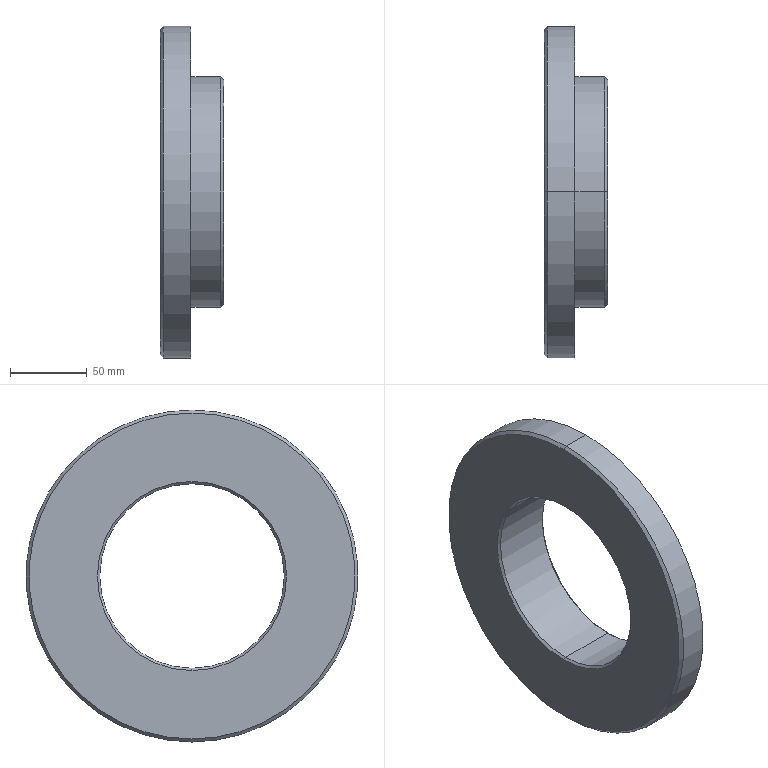Part | STEP file | Oil retaining ring | 1 solid | 17 faces | box 41.5 x 216 x 216 mm | volume 640315 mm3 | cone 8 | cylinder 6 | plane 3 | commonest cylinder face diameters 120 x2 150 x2 216 x2
STEP:
#1=CARTESIAN_POINT('',(0.,0.,0.));
#2=DIRECTION('',(0.,0.,1.));
#3=DIRECTION('',(1.,0.,0.));
#4=AXIS2_PLACEMENT_3D('',#1,#2,#3);
#5=CARTESIAN_POINT('',(39.5,0.,75.));
#6=VERTEX_POINT('',#5);
#7=CARTESIAN_POINT('',(39.5,0.,-75.));
#8=VERTEX_POINT('',#7);
#9=CARTESIAN_POINT('',(39.5,0.,0.));
#10=DIRECTION('',(-1.,0.,0.));
#11=DIRECTION('',(0.,0.,1.));
#12=AXIS2_PLACEMENT_3D('',#9,#10,#11);
#13=CIRCLE('',#12,75.);
#14=CARTESIAN_POINT('',(0.,0.,0.));
#15=DIRECTION('',(-1.,0.,0.));
#16=DIRECTION('',(0.,0.,1.));
#17=AXIS2_PLACEMENT_3D('',#14,#15,#16);
#18=CYLINDRICAL_SURFACE('',#17,75.);
#19=CARTESIAN_POINT('',(0.,-39.5));
#20=DIRECTION('',(1.,0.));
#21=VECTOR('',#20,1.);
#22=LINE('',#19,#21);
#23=(GEOMETRIC_REPRESENTATION_CONTEXT(2)PARAMETRIC_REPRESENTATION_CONTEXT()REPRESENTATION_CONTEXT('',''));
#24=DEFINITIONAL_REPRESENTATION('',(#22),#23);
#25=PCURVE('',#18,#24);
#26=CARTESIAN_POINT('',(41.5,0.,0.));
#27=DIRECTION('',(-1.,0.,0.));
#28=DIRECTION('',(0.,0.,1.));
#29=AXIS2_PLACEMENT_3D('',#26,#27,#28);
#30=CONICAL_SURFACE('',#29,73.,0.7854);
#31=CARTESIAN_POINT('',(0.,2.));
#32=DIRECTION('',(1.,0.));
#33=VECTOR('',#32,1.);
#34=LINE('',#31,#33);
#35=(GEOMETRIC_REPRESENTATION_CONTEXT(2)PARAMETRIC_REPRESENTATION_CONTEXT()REPRESENTATION_CONTEXT('',''));
#36=DEFINITIONAL_REPRESENTATION('',(#34),#35);
#37=PCURVE('',#30,#36);
#38=SURFACE_CURVE('',#13,(#25,#37),.PCURVE_S1.);
#39=EDGE_CURVE('',#6,#8,#38,.T.);
#40=ORIENTED_EDGE('',*,*,#39,.T.);
#41=CARTESIAN_POINT('',(20.,0.,-75.));
#42=VERTEX_POINT('',#41);
#43=CARTESIAN_POINT('',(0.,0.,-75.));
#44=DIRECTION('',(-1.,0.,0.));
#45=VECTOR('',#44,1.);
#46=LINE('',#43,#45);
#47=CARTESIAN_POINT('',(3.142,0.));
#48=DIRECTION('',(0.,1.));
#49=VECTOR('',#48,1.);
#50=LINE('',#47,#49);
#51=(GEOMETRIC_REPRESENTATION_CONTEXT(2)PARAMETRIC_REPRESENTATION_CONTEXT()REPRESENTATION_CONTEXT('',''));
#52=DEFINITIONAL_REPRESENTATION('',(#50),#51);
#53=PCURVE('',#18,#52);
#54=CARTESIAN_POINT('',(0.,0.,0.));
#55=DIRECTION('',(-1.,0.,0.));
#56=DIRECTION('',(0.,0.,1.));
#57=AXIS2_PLACEMENT_3D('',#54,#55,#56);
#58=CYLINDRICAL_SURFACE('',#57,75.);
#59=CARTESIAN_POINT('',(3.142,0.));
#60=DIRECTION('',(0.,1.));
#61=VECTOR('',#60,1.);
#62=LINE('',#59,#61);
#63=(GEOMETRIC_REPRESENTATION_CONTEXT(2)PARAMETRIC_REPRESENTATION_CONTEXT()REPRESENTATION_CONTEXT('',''));
#64=DEFINITIONAL_REPRESENTATION('',(#62),#63);
#65=PCURVE('',#58,#64);
#66=SURFACE_CURVE('',#46,(#53,#65),.PCURVE_S1.);
#67=EDGE_CURVE('',#8,#42,#66,.T.);
#68=ORIENTED_EDGE('',*,*,#67,.T.);
#69=CARTESIAN_POINT('',(20.,0.,75.));
#70=VERTEX_POINT('',#69);
#71=CARTESIAN_POINT('',(20.,0.,0.));
#72=DIRECTION('',(-1.,0.,0.));
#73=DIRECTION('',(0.,0.,1.));
#74=AXIS2_PLACEMENT_3D('',#71,#72,#73);
#75=CIRCLE('',#74,75.);
#76=CARTESIAN_POINT('',(0.,-20.));
#77=DIRECTION('',(1.,0.));
#78=VECTOR('',#77,1.);
#79=LINE('',#76,#78);
#80=(GEOMETRIC_REPRESENTATION_CONTEXT(2)PARAMETRIC_REPRESENTATION_CONTEXT()REPRESENTATION_CONTEXT('',''));
#81=DEFINITIONAL_REPRESENTATION('',(#79),#80);
#82=PCURVE('',#18,#81);
#83=CARTESIAN_POINT('',(20.,108.,0.));
#84=DIRECTION('',(-1.,0.,0.));
#85=DIRECTION('',(0.,0.,1.));
#86=AXIS2_PLACEMENT_3D('',#83,#84,#85);
#87=PLANE('',#86);
#88=CARTESIAN_POINT('',(0.,-108.));
#89=DIRECTION('',(1.,0.));
#90=AXIS2_PLACEMENT_2D('',#88,#89);
#91=CIRCLE('',#90,75.);
#92=(GEOMETRIC_REPRESENTATION_CONTEXT(2)PARAMETRIC_REPRESENTATION_CONTEXT()REPRESENTATION_CONTEXT('',''));
#93=DEFINITIONAL_REPRESENTATION('',(#91),#92);
#94=PCURVE('',#87,#93);
#95=SURFACE_CURVE('',#75,(#82,#94),.PCURVE_S1.);
#96=EDGE_CURVE('',#70,#42,#95,.T.);
#97=ORIENTED_EDGE('',*,*,#96,.F.);
#98=CARTESIAN_POINT('',(0.,0.,75.));
#99=DIRECTION('',(-1.,0.,0.));
#100=VECTOR('',#99,1.);
#101=LINE('',#98,#100);
#102=CARTESIAN_POINT('',(0.,0.));
#103=DIRECTION('',(0.,1.));
#104=VECTOR('',#103,1.);
#105=LINE('',#102,#104);
#106=(GEOMETRIC_REPRESENTATION_CONTEXT(2)PARAMETRIC_REPRESENTATION_CONTEXT()REPRESENTATION_CONTEXT('',''));
#107=DEFINITIONAL_REPRESENTATION('',(#105),#106);
#108=PCURVE('',#18,#107);
#109=CARTESIAN_POINT('',(6.283,0.));
#110=DIRECTION('',(0.,1.));
#111=VECTOR('',#110,1.);
#112=LINE('',#109,#111);
#113=(GEOMETRIC_REPRESENTATION_CONTEXT(2)PARAMETRIC_REPRESENTATION_CONTEXT()REPRESENTATION_CONTEXT('',''));
#114=DEFINITIONAL_REPRESENTATION('',(#112),#113);
#115=PCURVE('',#58,#114);
#116=SURFACE_CURVE('',#101,(#108,#115),.PCURVE_S1.);
#117=EDGE_CURVE('',#6,#70,#116,.T.);
#118=ORIENTED_EDGE('',*,*,#117,.F.);
#119=EDGE_LOOP('',(#40,#68,#97,#118));
#120=FACE_BOUND('',#119,.T.);
#121=ADVANCED_FACE('',(#120),#18,.T.);
#122=CARTESIAN_POINT('',(20.,0.,108.));
#123=VERTEX_POINT('',#122);
#124=CARTESIAN_POINT('',(20.,0.,-108.));
#125=VERTEX_POINT('',#124);
#126=CARTESIAN_POINT('',(20.,0.,0.));
#127=DIRECTION('',(-1.,0.,0.));
#128=DIRECTION('',(0.,0.,1.));
#129=AXIS2_PLACEMENT_3D('',#126,#127,#128);
#130=CIRCLE('',#129,108.);
#131=CARTESIAN_POINT('',(0.,0.,0.));
#132=DIRECTION('',(-1.,0.,0.));
#133=DIRECTION('',(0.,0.,1.));
#134=AXIS2_PLACEMENT_3D('',#131,#132,#133);
#135=CYLINDRICAL_SURFACE('',#134,108.);
#136=CARTESIAN_POINT('',(0.,-20.));
#137=DIRECTION('',(1.,0.));
#138=VECTOR('',#137,1.);
#139=LINE('',#136,#138);
#140=(GEOMETRIC_REPRESENTATION_CONTEXT(2)PARAMETRIC_REPRESENTATION_CONTEXT()REPRESENTATION_CONTEXT('',''));
#141=DEFINITIONAL_REPRESENTATION('',(#139),#140);
#142=PCURVE('',#135,#141);
#143=CARTESIAN_POINT('',(0.,-108.));
#144=DIRECTION('',(1.,0.));
#145=AXIS2_PLACEMENT_2D('',#143,#144);
#146=CIRCLE('',#145,108.);
#147=(GEOMETRIC_REPRESENTATION_CONTEXT(2)PARAMETRIC_REPRESENTATION_CONTEXT()REPRESENTATION_CONTEXT('',''));
#148=DEFINITIONAL_REPRESENTATION('',(#146),#147);
#149=PCURVE('',#87,#148);
#150=SURFACE_CURVE('',#130,(#142,#149),.PCURVE_S1.);
#151=EDGE_CURVE('',#123,#125,#150,.T.);
#152=ORIENTED_EDGE('',*,*,#151,.T.);
#153=CARTESIAN_POINT('',(2.,0.,-108.));
#154=VERTEX_POINT('',#153);
#155=CARTESIAN_POINT('',(0.,0.,-108.));
#156=DIRECTION('',(-1.,0.,0.));
#157=VECTOR('',#156,1.);
#158=LINE('',#155,#157);
#159=CARTESIAN_POINT('',(3.142,0.));
#160=DIRECTION('',(0.,1.));
#161=VECTOR('',#160,1.);
#162=LINE('',#159,#161);
#163=(GEOMETRIC_REPRESENTATION_CONTEXT(2)PARAMETRIC_REPRESENTATION_CONTEXT()REPRESENTATION_CONTEXT('',''));
#164=DEFINITIONAL_REPRESENTATION('',(#162),#163);
#165=PCURVE('',#135,#164);
#166=CARTESIAN_POINT('',(0.,0.,0.));
#167=DIRECTION('',(-1.,0.,0.));
#168=DIRECTION('',(0.,0.,1.));
#169=AXIS2_PLACEMENT_3D('',#166,#167,#168);
#170=CYLINDRICAL_SURFACE('',#169,108.);
#171=CARTESIAN_POINT('',(3.142,0.));
#172=DIRECTION('',(0.,1.));
#173=VECTOR('',#172,1.);
#174=LINE('',#171,#173);
#175=(GEOMETRIC_REPRESENTATION_CONTEXT(2)PARAMETRIC_REPRESENTATION_CONTEXT()REPRESENTATION_CONTEXT('',''));
#176=DEFINITIONAL_REPRESENTATION('',(#174),#175);
#177=PCURVE('',#170,#176);
#178=SURFACE_CURVE('',#158,(#165,#177),.PCURVE_S1.);
#179=EDGE_CURVE('',#125,#154,#178,.T.);
#180=ORIENTED_EDGE('',*,*,#179,.T.);
#181=CARTESIAN_POINT('',(2.,0.,108.));
#182=VERTEX_POINT('',#181);
#183=CARTESIAN_POINT('',(2.,0.,0.));
#184=DIRECTION('',(-1.,0.,0.));
#185=DIRECTION('',(0.,0.,1.));
#186=AXIS2_PLACEMENT_3D('',#183,#184,#185);
#187=CIRCLE('',#186,108.);
#188=CARTESIAN_POINT('',(0.,-2.));
#189=DIRECTION('',(1.,0.));
#190=VECTOR('',#189,1.);
#191=LINE('',#188,#190);
#192=(GEOMETRIC_REPRESENTATION_CONTEXT(2)PARAMETRIC_REPRESENTATION_CONTEXT()REPRESENTATION_CONTEXT('',''));
#193=DEFINITIONAL_REPRESENTATION('',(#191),#192);
#194=PCURVE('',#135,#193);
#195=CARTESIAN_POINT('',(2.,0.,0.));
#196=DIRECTION('',(1.,0.,0.));
#197=DIRECTION('',(0.,0.,-1.));
#198=AXIS2_PLACEMENT_3D('',#195,#196,#197);
#199=CONICAL_SURFACE('',#198,108.,0.7854);
#200=CARTESIAN_POINT('',(3.142,0.));
#201=DIRECTION('',(-1.,0.));
#202=VECTOR('',#201,1.);
#203=LINE('',#200,#202);
#204=(GEOMETRIC_REPRESENTATION_CONTEXT(2)PARAMETRIC_REPRESENTATION_CONTEXT()REPRESENTATION_CONTEXT('',''));
#205=DEFINITIONAL_REPRESENTATION('',(#203),#204);
#206=PCURVE('',#199,#205);
#207=SURFACE_CURVE('',#187,(#194,#206),.PCURVE_S1.);
#208=EDGE_CURVE('',#182,#154,#207,.T.);
#209=ORIENTED_EDGE('',*,*,#208,.F.);
#210=CARTESIAN_POINT('',(0.,0.,108.));
#211=DIRECTION('',(-1.,0.,0.));
#212=VECTOR('',#211,1.);
#213=LINE('',#210,#212);
#214=CARTESIAN_POINT('',(0.,0.));
#215=DIRECTION('',(0.,1.));
#216=VECTOR('',#215,1.);
#217=LINE('',#214,#216);
#218=(GEOMETRIC_REPRESENTATION_CONTEXT(2)PARAMETRIC_REPRESENTATION_CONTEXT()REPRESENTATION_CONTEXT('',''));
#219=DEFINITIONAL_REPRESENTATION('',(#217),#218);
#220=PCURVE('',#135,#219);
#221=CARTESIAN_POINT('',(6.283,0.));
#222=DIRECTION('',(0.,1.));
#223=VECTOR('',#222,1.);
#224=LINE('',#221,#223);
#225=(GEOMETRIC_REPRESENTATION_CONTEXT(2)PARAMETRIC_REPRESENTATION_CONTEXT()REPRESENTATION_CONTEXT('',''));
#226=DEFINITIONAL_REPRESENTATION('',(#224),#225);
#227=PCURVE('',#170,#226);
#228=SURFACE_CURVE('',#213,(#220,#227),.PCURVE_S1.);
#229=EDGE_CURVE('',#123,#182,#228,.T.);
#230=ORIENTED_EDGE('',*,*,#229,.F.);
#231=EDGE_LOOP('',(#152,#180,#209,#230));
#232=FACE_BOUND('',#231,.T.);
#233=ADVANCED_FACE('',(#232),#135,.T.);
#234=CARTESIAN_POINT('',(0.,0.,106.));
#235=VERTEX_POINT('',#234);
#236=CARTESIAN_POINT('',(0.,0.,-106.));
#237=VERTEX_POINT('',#236);
#238=CARTESIAN_POINT('',(0.,0.,0.));
#239=DIRECTION('',(-1.,0.,0.));
#240=DIRECTION('',(0.,0.,1.));
#241=AXIS2_PLACEMENT_3D('',#238,#239,#240);
#242=CIRCLE('',#241,106.);
#243=CARTESIAN_POINT('',(3.142,-2.));
#244=DIRECTION('',(-1.,0.));
#245=VECTOR('',#244,1.);
#246=LINE('',#243,#245);
#247=(GEOMETRIC_REPRESENTATION_CONTEXT(2)PARAMETRIC_REPRESENTATION_CONTEXT()REPRESENTATION_CONTEXT('',''));
#248=DEFINITIONAL_REPRESENTATION('',(#246),#247);
#249=PCURVE('',#199,#248);
#250=CARTESIAN_POINT('',(0.,61.5,0.));
#251=DIRECTION('',(1.,0.,0.));
#252=DIRECTION('',(0.,0.,-1.));
#253=AXIS2_PLACEMENT_3D('',#250,#251,#252);
#254=PLANE('',#253);
#255=CARTESIAN_POINT('',(-106.,-61.5));
#256=CARTESIAN_POINT('',(-106.,122.097));
#257=CARTESIAN_POINT('',(53.,30.299));
#258=CARTESIAN_POINT('',(212.,-61.5));
#259=CARTESIAN_POINT('',(53.,-153.299));
#260=CARTESIAN_POINT('',(-106.,-245.097));
#261=CARTESIAN_POINT('',(-106.,-61.5));
#262=(BOUNDED_CURVE()B_SPLINE_CURVE(2,(#255,#256,#257,#258,#259,#260,#261),.UNSPECIFIED.,.T.,.F.)B_SPLINE_CURVE_WITH_KNOTS((1,2,2,2,2,1),(-2.094,0.,2.094,4.189,6.283,8.378),.UNSPECIFIED.)CURVE()GEOMETRIC_REPRESENTATION_ITEM()RATIONAL_B_SPLINE_CURVE((1.,0.5,1.,0.5,1.,0.5,1.))REPRESENTATION_ITEM(''));
#263=(GEOMETRIC_REPRESENTATION_CONTEXT(2)PARAMETRIC_REPRESENTATION_CONTEXT()REPRESENTATION_CONTEXT('',''));
#264=DEFINITIONAL_REPRESENTATION('',(#262),#263);
#265=PCURVE('',#254,#264);
#266=SURFACE_CURVE('',#242,(#249,#265),.PCURVE_S1.);
#267=EDGE_CURVE('',#235,#237,#266,.T.);
#268=ORIENTED_EDGE('',*,*,#267,.F.);
#269=CARTESIAN_POINT('',(2.,0.,108.));
#270=DIRECTION('',(0.7071,0.,0.7071));
#271=VECTOR('',#270,1.);
#272=LINE('',#269,#271);
#273=CARTESIAN_POINT('',(3.142,0.));
#274=DIRECTION('',(0.,1.));
#275=VECTOR('',#274,1.);
#276=LINE('',#273,#275);
#277=(GEOMETRIC_REPRESENTATION_CONTEXT(2)PARAMETRIC_REPRESENTATION_CONTEXT()REPRESENTATION_CONTEXT('',''));
#278=DEFINITIONAL_REPRESENTATION('',(#276),#277);
#279=PCURVE('',#199,#278);
#280=CARTESIAN_POINT('',(2.,0.,0.));
#281=DIRECTION('',(1.,0.,0.));
#282=DIRECTION('',(0.,0.,-1.));
#283=AXIS2_PLACEMENT_3D('',#280,#281,#282);
#284=CONICAL_SURFACE('',#283,108.,0.7854);
#285=CARTESIAN_POINT('',(3.142,0.));
#286=DIRECTION('',(0.,1.));
#287=VECTOR('',#286,1.);
#288=LINE('',#285,#287);
#289=(GEOMETRIC_REPRESENTATION_CONTEXT(2)PARAMETRIC_REPRESENTATION_CONTEXT()REPRESENTATION_CONTEXT('',''));
#290=DEFINITIONAL_REPRESENTATION('',(#288),#289);
#291=PCURVE('',#284,#290);
#292=SURFACE_CURVE('',#272,(#279,#291),.PCURVE_S1.);
#293=EDGE_CURVE('',#235,#182,#292,.T.);
#294=ORIENTED_EDGE('',*,*,#293,.T.);
#295=ORIENTED_EDGE('',*,*,#208,.T.);
#296=CARTESIAN_POINT('',(2.,0.,-108.));
#297=DIRECTION('',(0.7071,0.,-0.7071));
#298=VECTOR('',#297,1.);
#299=LINE('',#296,#298);
#300=CARTESIAN_POINT('',(0.,0.));
#301=DIRECTION('',(0.,1.));
#302=VECTOR('',#301,1.);
#303=LINE('',#300,#302);
#304=(GEOMETRIC_REPRESENTATION_CONTEXT(2)PARAMETRIC_REPRESENTATION_CONTEXT()REPRESENTATION_CONTEXT('',''));
#305=DEFINITIONAL_REPRESENTATION('',(#303),#304);
#306=PCURVE('',#199,#305);
#307=CARTESIAN_POINT('',(6.283,0.));
#308=DIRECTION('',(0.,1.));
#309=VECTOR('',#308,1.);
#310=LINE('',#307,#309);
#311=(GEOMETRIC_REPRESENTATION_CONTEXT(2)PARAMETRIC_REPRESENTATION_CONTEXT()REPRESENTATION_CONTEXT('',''));
#312=DEFINITIONAL_REPRESENTATION('',(#310),#311);
#313=PCURVE('',#284,#312);
#314=SURFACE_CURVE('',#299,(#306,#313),.PCURVE_S1.);
#315=EDGE_CURVE('',#237,#154,#314,.T.);
#316=ORIENTED_EDGE('',*,*,#315,.F.);
#317=EDGE_LOOP('',(#268,#294,#295,#316));
#318=FACE_BOUND('',#317,.T.);
#319=ADVANCED_FACE('',(#318),#199,.T.);
#320=CARTESIAN_POINT('',(1.5,0.,60.));
#321=VERTEX_POINT('',#320);
#322=CARTESIAN_POINT('',(0.,0.,61.5));
#323=VERTEX_POINT('',#322);
#324=CARTESIAN_POINT('',(0.,0.,61.5));
#325=DIRECTION('',(-0.7071,0.,0.7071));
#326=VECTOR('',#325,1.);
#327=LINE('',#324,#326);
#328=CARTESIAN_POINT('',(0.,0.,0.));
#329=DIRECTION('',(-1.,0.,0.));
#330=DIRECTION('',(0.,0.,1.));
#331=AXIS2_PLACEMENT_3D('',#328,#329,#330);
#332=CONICAL_SURFACE('',#331,61.5,0.7854);
#333=CARTESIAN_POINT('',(6.283,0.));
#334=DIRECTION('',(0.,1.));
#335=VECTOR('',#334,1.);
#336=LINE('',#333,#335);
#337=(GEOMETRIC_REPRESENTATION_CONTEXT(2)PARAMETRIC_REPRESENTATION_CONTEXT()REPRESENTATION_CONTEXT('',''));
#338=DEFINITIONAL_REPRESENTATION('',(#336),#337);
#339=PCURVE('',#332,#338);
#340=CARTESIAN_POINT('',(0.,0.,0.));
#341=DIRECTION('',(-1.,0.,0.));
#342=DIRECTION('',(0.,0.,1.));
#343=AXIS2_PLACEMENT_3D('',#340,#341,#342);
#344=CONICAL_SURFACE('',#343,61.5,0.7854);
#345=CARTESIAN_POINT('',(0.,0.));
#346=DIRECTION('',(0.,1.));
#347=VECTOR('',#346,1.);
#348=LINE('',#345,#347);
#349=(GEOMETRIC_REPRESENTATION_CONTEXT(2)PARAMETRIC_REPRESENTATION_CONTEXT()REPRESENTATION_CONTEXT('',''));
#350=DEFINITIONAL_REPRESENTATION('',(#348),#349);
#351=PCURVE('',#344,#350);
#352=SURFACE_CURVE('',#327,(#339,#351),.PCURVE_S1.);
#353=EDGE_CURVE('',#321,#323,#352,.T.);
#354=ORIENTED_EDGE('',*,*,#353,.T.);
#355=CARTESIAN_POINT('',(0.,0.,-61.5));
#356=VERTEX_POINT('',#355);
#357=CARTESIAN_POINT('',(0.,0.,0.));
#358=DIRECTION('',(-1.,0.,0.));
#359=DIRECTION('',(0.,0.,1.));
#360=AXIS2_PLACEMENT_3D('',#357,#358,#359);
#361=CIRCLE('',#360,61.5);
#362=CARTESIAN_POINT('',(0.,0.));
#363=DIRECTION('',(1.,0.));
#364=VECTOR('',#363,1.);
#365=LINE('',#362,#364);
#366=(GEOMETRIC_REPRESENTATION_CONTEXT(2)PARAMETRIC_REPRESENTATION_CONTEXT()REPRESENTATION_CONTEXT('',''));
#367=DEFINITIONAL_REPRESENTATION('',(#365),#366);
#368=PCURVE('',#332,#367);
#369=CARTESIAN_POINT('',(-61.5,-61.5));
#370=CARTESIAN_POINT('',(-61.5,45.021));
#371=CARTESIAN_POINT('',(30.75,-8.239));
#372=CARTESIAN_POINT('',(123.,-61.5));
#373=CARTESIAN_POINT('',(30.75,-114.761));
#374=CARTESIAN_POINT('',(-61.5,-168.021));
#375=CARTESIAN_POINT('',(-61.5,-61.5));
#376=(BOUNDED_CURVE()B_SPLINE_CURVE(2,(#369,#370,#371,#372,#373,#374,#375),.UNSPECIFIED.,.T.,.F.)B_SPLINE_CURVE_WITH_KNOTS((1,2,2,2,2,1),(-2.094,0.,2.094,4.189,6.283,8.378),.UNSPECIFIED.)CURVE()GEOMETRIC_REPRESENTATION_ITEM()RATIONAL_B_SPLINE_CURVE((1.,0.5,1.,0.5,1.,0.5,1.))REPRESENTATION_ITEM(''));
#377=(GEOMETRIC_REPRESENTATION_CONTEXT(2)PARAMETRIC_REPRESENTATION_CONTEXT()REPRESENTATION_CONTEXT('',''));
#378=DEFINITIONAL_REPRESENTATION('',(#376),#377);
#379=PCURVE('',#254,#378);
#380=SURFACE_CURVE('',#361,(#368,#379),.PCURVE_S1.);
#381=EDGE_CURVE('',#356,#323,#380,.T.);
#382=ORIENTED_EDGE('',*,*,#381,.F.);
#383=CARTESIAN_POINT('',(1.5,0.,-60.));
#384=VERTEX_POINT('',#383);
#385=CARTESIAN_POINT('',(0.,0.,-61.5));
#386=DIRECTION('',(-0.7071,0.,-0.7071));
#387=VECTOR('',#386,1.);
#388=LINE('',#385,#387);
#389=CARTESIAN_POINT('',(3.142,0.));
#390=DIRECTION('',(0.,1.));
#391=VECTOR('',#390,1.);
#392=LINE('',#389,#391);
#393=(GEOMETRIC_REPRESENTATION_CONTEXT(2)PARAMETRIC_REPRESENTATION_CONTEXT()REPRESENTATION_CONTEXT('',''));
#394=DEFINITIONAL_REPRESENTATION('',(#392),#393);
#395=PCURVE('',#332,#394);
#396=CARTESIAN_POINT('',(3.142,0.));
#397=DIRECTION('',(0.,1.));
#398=VECTOR('',#397,1.);
#399=LINE('',#396,#398);
#400=(GEOMETRIC_REPRESENTATION_CONTEXT(2)PARAMETRIC_REPRESENTATION_CONTEXT()REPRESENTATION_CONTEXT('',''));
#401=DEFINITIONAL_REPRESENTATION('',(#399),#400);
#402=PCURVE('',#344,#401);
#403=SURFACE_CURVE('',#388,(#395,#402),.PCURVE_S1.);
#404=EDGE_CURVE('',#384,#356,#403,.T.);
#405=ORIENTED_EDGE('',*,*,#404,.F.);
#406=CARTESIAN_POINT('',(1.5,0.,0.));
#407=DIRECTION('',(-1.,0.,0.));
#408=DIRECTION('',(0.,0.,1.));
#409=AXIS2_PLACEMENT_3D('',#406,#407,#408);
#410=CIRCLE('',#409,60.);
#411=CARTESIAN_POINT('',(0.,-1.5));
#412=DIRECTION('',(1.,0.));
#413=VECTOR('',#412,1.);
#414=LINE('',#411,#413);
#415=(GEOMETRIC_REPRESENTATION_CONTEXT(2)PARAMETRIC_REPRESENTATION_CONTEXT()REPRESENTATION_CONTEXT('',''));
#416=DEFINITIONAL_REPRESENTATION('',(#414),#415);
#417=PCURVE('',#332,#416);
#418=CARTESIAN_POINT('',(0.,0.,0.));
#419=DIRECTION('',(-1.,0.,0.));
#420=DIRECTION('',(0.,0.,1.));
#421=AXIS2_PLACEMENT_3D('',#418,#419,#420);
#422=CYLINDRICAL_SURFACE('',#421,60.);
#423=CARTESIAN_POINT('',(0.,-1.5));
#424=DIRECTION('',(1.,0.));
#425=VECTOR('',#424,1.);
#426=LINE('',#423,#425);
#427=(GEOMETRIC_REPRESENTATION_CONTEXT(2)PARAMETRIC_REPRESENTATION_CONTEXT()REPRESENTATION_CONTEXT('',''));
#428=DEFINITIONAL_REPRESENTATION('',(#426),#427);
#429=PCURVE('',#422,#428);
#430=SURFACE_CURVE('',#410,(#417,#429),.PCURVE_S1.);
#431=EDGE_CURVE('',#384,#321,#430,.T.);
#432=ORIENTED_EDGE('',*,*,#431,.T.);
#433=EDGE_LOOP('',(#354,#382,#405,#432));
#434=FACE_BOUND('',#433,.F.);
#435=ADVANCED_FACE('',(#434),#332,.F.);
#436=CARTESIAN_POINT('',(40.,0.,60.));
#437=VERTEX_POINT('',#436);
#438=CARTESIAN_POINT('',(0.,0.,60.));
#439=DIRECTION('',(-1.,0.,0.));
#440=VECTOR('',#439,1.);
#441=LINE('',#438,#440);
#442=CARTESIAN_POINT('',(6.283,0.));
#443=DIRECTION('',(0.,1.));
#444=VECTOR('',#443,1.);
#445=LINE('',#442,#444);
#446=(GEOMETRIC_REPRESENTATION_CONTEXT(2)PARAMETRIC_REPRESENTATION_CONTEXT()REPRESENTATION_CONTEXT('',''));
#447=DEFINITIONAL_REPRESENTATION('',(#445),#446);
#448=PCURVE('',#422,#447);
#449=CARTESIAN_POINT('',(0.,0.,0.));
#450=DIRECTION('',(-1.,0.,0.));
#451=DIRECTION('',(0.,0.,1.));
#452=AXIS2_PLACEMENT_3D('',#449,#450,#451);
#453=CYLINDRICAL_SURFACE('',#452,60.);
#454=CARTESIAN_POINT('',(0.,0.));
#455=DIRECTION('',(0.,1.));
#456=VECTOR('',#455,1.);
#457=LINE('',#454,#456);
#458=(GEOMETRIC_REPRESENTATION_CONTEXT(2)PARAMETRIC_REPRESENTATION_CONTEXT()REPRESENTATION_CONTEXT('',''));
#459=DEFINITIONAL_REPRESENTATION('',(#457),#458);
#460=PCURVE('',#453,#459);
#461=SURFACE_CURVE('',#441,(#448,#460),.PCURVE_S1.);
#462=EDGE_CURVE('',#437,#321,#461,.T.);
#463=ORIENTED_EDGE('',*,*,#462,.T.);
#464=ORIENTED_EDGE('',*,*,#431,.F.);
#465=CARTESIAN_POINT('',(40.,0.,-60.));
#466=VERTEX_POINT('',#465);
#467=CARTESIAN_POINT('',(0.,0.,-60.));
#468=DIRECTION('',(-1.,0.,0.));
#469=VECTOR('',#468,1.);
#470=LINE('',#467,#469);
#471=CARTESIAN_POINT('',(3.142,0.));
#472=DIRECTION('',(0.,1.));
#473=VECTOR('',#472,1.);
#474=LINE('',#471,#473);
#475=(GEOMETRIC_REPRESENTATION_CONTEXT(2)PARAMETRIC_REPRESENTATION_CONTEXT()REPRESENTATION_CONTEXT('',''));
#476=DEFINITIONAL_REPRESENTATION('',(#474),#475);
#477=PCURVE('',#422,#476);
#478=CARTESIAN_POINT('',(3.142,0.));
#479=DIRECTION('',(0.,1.));
#480=VECTOR('',#479,1.);
#481=LINE('',#478,#480);
#482=(GEOMETRIC_REPRESENTATION_CONTEXT(2)PARAMETRIC_REPRESENTATION_CONTEXT()REPRESENTATION_CONTEXT('',''));
#483=DEFINITIONAL_REPRESENTATION('',(#481),#482);
#484=PCURVE('',#453,#483);
#485=SURFACE_CURVE('',#470,(#477,#484),.PCURVE_S1.);
#486=EDGE_CURVE('',#466,#384,#485,.T.);
#487=ORIENTED_EDGE('',*,*,#486,.F.);
#488=CARTESIAN_POINT('',(40.,0.,0.));
#489=DIRECTION('',(-1.,0.,0.));
#490=DIRECTION('',(0.,0.,1.));
#491=AXIS2_PLACEMENT_3D('',#488,#489,#490);
#492=CIRCLE('',#491,60.);
#493=CARTESIAN_POINT('',(0.,-40.));
#494=DIRECTION('',(1.,0.));
#495=VECTOR('',#494,1.);
#496=LINE('',#493,#495);
#497=(GEOMETRIC_REPRESENTATION_CONTEXT(2)PARAMETRIC_REPRESENTATION_CONTEXT()REPRESENTATION_CONTEXT('',''));
#498=DEFINITIONAL_REPRESENTATION('',(#496),#497);
#499=PCURVE('',#422,#498);
#500=CARTESIAN_POINT('',(40.,0.,0.));
#501=DIRECTION('',(1.,0.,0.));
#502=DIRECTION('',(0.,0.,-1.));
#503=AXIS2_PLACEMENT_3D('',#500,#501,#502);
#504=CONICAL_SURFACE('',#503,60.,0.7854);
#505=CARTESIAN_POINT('',(9.425,0.));
#506=DIRECTION('',(-1.,0.));
#507=VECTOR('',#506,1.);
#508=LINE('',#505,#507);
#509=(GEOMETRIC_REPRESENTATION_CONTEXT(2)PARAMETRIC_REPRESENTATION_CONTEXT()REPRESENTATION_CONTEXT('',''));
#510=DEFINITIONAL_REPRESENTATION('',(#508),#509);
#511=PCURVE('',#504,#510);
#512=SURFACE_CURVE('',#492,(#499,#511),.PCURVE_S1.);
#513=EDGE_CURVE('',#466,#437,#512,.T.);
#514=ORIENTED_EDGE('',*,*,#513,.T.);
#515=EDGE_LOOP('',(#463,#464,#487,#514));
#516=FACE_BOUND('',#515,.F.);
#517=ADVANCED_FACE('',(#516),#422,.F.);
#518=CARTESIAN_POINT('',(41.5,0.,-61.5));
#519=VERTEX_POINT('',#518);
#520=CARTESIAN_POINT('',(40.,0.,-60.));
#521=DIRECTION('',(0.7071,0.,-0.7071));
#522=VECTOR('',#521,1.);
#523=LINE('',#520,#522);
#524=CARTESIAN_POINT('',(6.283,0.));
#525=DIRECTION('',(0.,1.));
#526=VECTOR('',#525,1.);
#527=LINE('',#524,#526);
#528=(GEOMETRIC_REPRESENTATION_CONTEXT(2)PARAMETRIC_REPRESENTATION_CONTEXT()REPRESENTATION_CONTEXT('',''));
#529=DEFINITIONAL_REPRESENTATION('',(#527),#528);
#530=PCURVE('',#504,#529);
#531=CARTESIAN_POINT('',(40.,0.,0.));
#532=DIRECTION('',(1.,0.,0.));
#533=DIRECTION('',(0.,0.,-1.));
#534=AXIS2_PLACEMENT_3D('',#531,#532,#533);
#535=CONICAL_SURFACE('',#534,60.,0.7854);
#536=CARTESIAN_POINT('',(0.,0.));
#537=DIRECTION('',(0.,1.));
#538=VECTOR('',#537,1.);
#539=LINE('',#536,#538);
#540=(GEOMETRIC_REPRESENTATION_CONTEXT(2)PARAMETRIC_REPRESENTATION_CONTEXT()REPRESENTATION_CONTEXT('',''));
#541=DEFINITIONAL_REPRESENTATION('',(#539),#540);
#542=PCURVE('',#535,#541);
#543=SURFACE_CURVE('',#523,(#530,#542),.PCURVE_S1.);
#544=EDGE_CURVE('',#466,#519,#543,.T.);
#545=ORIENTED_EDGE('',*,*,#544,.T.);
#546=CARTESIAN_POINT('',(41.5,0.,61.5));
#547=VERTEX_POINT('',#546);
#548=CARTESIAN_POINT('',(41.5,0.,0.));
#549=DIRECTION('',(-1.,0.,0.));
#550=DIRECTION('',(0.,0.,1.));
#551=AXIS2_PLACEMENT_3D('',#548,#549,#550);
#552=CIRCLE('',#551,61.5);
#553=CARTESIAN_POINT('',(9.425,1.5));
#554=DIRECTION('',(-1.,0.));
#555=VECTOR('',#554,1.);
#556=LINE('',#553,#555);
#557=(GEOMETRIC_REPRESENTATION_CONTEXT(2)PARAMETRIC_REPRESENTATION_CONTEXT()REPRESENTATION_CONTEXT('',''));
#558=DEFINITIONAL_REPRESENTATION('',(#556),#557);
#559=PCURVE('',#504,#558);
#560=CARTESIAN_POINT('',(41.5,73.,0.));
#561=DIRECTION('',(-1.,0.,0.));
#562=DIRECTION('',(0.,0.,1.));
#563=AXIS2_PLACEMENT_3D('',#560,#561,#562);
#564=PLANE('',#563);
#565=CARTESIAN_POINT('',(0.,-73.));
#566=DIRECTION('',(1.,0.));
#567=AXIS2_PLACEMENT_2D('',#565,#566);
#568=CIRCLE('',#567,61.5);
#569=(GEOMETRIC_REPRESENTATION_CONTEXT(2)PARAMETRIC_REPRESENTATION_CONTEXT()REPRESENTATION_CONTEXT('',''));
#570=DEFINITIONAL_REPRESENTATION('',(#568),#569);
#571=PCURVE('',#564,#570);
#572=SURFACE_CURVE('',#552,(#559,#571),.PCURVE_S1.);
#573=EDGE_CURVE('',#519,#547,#572,.T.);
#574=ORIENTED_EDGE('',*,*,#573,.T.);
#575=CARTESIAN_POINT('',(40.,0.,60.));
#576=DIRECTION('',(0.7071,0.,0.7071));
#577=VECTOR('',#576,1.);
#578=LINE('',#575,#577);
#579=CARTESIAN_POINT('',(3.142,0.));
#580=DIRECTION('',(0.,1.));
#581=VECTOR('',#580,1.);
#582=LINE('',#579,#581);
#583=(GEOMETRIC_REPRESENTATION_CONTEXT(2)PARAMETRIC_REPRESENTATION_CONTEXT()REPRESENTATION_CONTEXT('',''));
#584=DEFINITIONAL_REPRESENTATION('',(#582),#583);
#585=PCURVE('',#504,#584);
#586=CARTESIAN_POINT('',(3.142,0.));
#587=DIRECTION('',(0.,1.));
#588=VECTOR('',#587,1.);
#589=LINE('',#586,#588);
#590=(GEOMETRIC_REPRESENTATION_CONTEXT(2)PARAMETRIC_REPRESENTATION_CONTEXT()REPRESENTATION_CONTEXT('',''));
#591=DEFINITIONAL_REPRESENTATION('',(#589),#590);
#592=PCURVE('',#535,#591);
#593=SURFACE_CURVE('',#578,(#585,#592),.PCURVE_S1.);
#594=EDGE_CURVE('',#437,#547,#593,.T.);
#595=ORIENTED_EDGE('',*,*,#594,.F.);
#596=ORIENTED_EDGE('',*,*,#513,.F.);
#597=EDGE_LOOP('',(#545,#574,#595,#596));
#598=FACE_BOUND('',#597,.F.);
#599=ADVANCED_FACE('',(#598),#504,.F.);
#600=CARTESIAN_POINT('',(41.5,0.,73.));
#601=VERTEX_POINT('',#600);
#602=CARTESIAN_POINT('',(41.5,0.,-73.));
#603=VERTEX_POINT('',#602);
#604=CARTESIAN_POINT('',(41.5,0.,0.));
#605=DIRECTION('',(-1.,0.,0.));
#606=DIRECTION('',(0.,0.,1.));
#607=AXIS2_PLACEMENT_3D('',#604,#605,#606);
#608=CIRCLE('',#607,73.);
#609=CARTESIAN_POINT('',(0.,0.));
#610=DIRECTION('',(1.,0.));
#611=VECTOR('',#610,1.);
#612=LINE('',#609,#611);
#613=(GEOMETRIC_REPRESENTATION_CONTEXT(2)PARAMETRIC_REPRESENTATION_CONTEXT()REPRESENTATION_CONTEXT('',''));
#614=DEFINITIONAL_REPRESENTATION('',(#612),#613);
#615=PCURVE('',#30,#614);
#616=CARTESIAN_POINT('',(0.,-73.));
#617=DIRECTION('',(1.,0.));
#618=AXIS2_PLACEMENT_2D('',#616,#617);
#619=CIRCLE('',#618,73.);
#620=(GEOMETRIC_REPRESENTATION_CONTEXT(2)PARAMETRIC_REPRESENTATION_CONTEXT()REPRESENTATION_CONTEXT('',''));
#621=DEFINITIONAL_REPRESENTATION('',(#619),#620);
#622=PCURVE('',#564,#621);
#623=SURFACE_CURVE('',#608,(#615,#622),.PCURVE_S1.);
#624=EDGE_CURVE('',#601,#603,#623,.T.);
#625=ORIENTED_EDGE('',*,*,#624,.T.);
#626=CARTESIAN_POINT('',(41.5,0.,-73.));
#627=DIRECTION('',(-0.7071,0.,-0.7071));
#628=VECTOR('',#627,1.);
#629=LINE('',#626,#628);
#630=CARTESIAN_POINT('',(3.142,0.));
#631=DIRECTION('',(0.,1.));
#632=VECTOR('',#631,1.);
#633=LINE('',#630,#632);
#634=(GEOMETRIC_REPRESENTATION_CONTEXT(2)PARAMETRIC_REPRESENTATION_CONTEXT()REPRESENTATION_CONTEXT('',''));
#635=DEFINITIONAL_REPRESENTATION('',(#633),#634);
#636=PCURVE('',#30,#635);
#637=CARTESIAN_POINT('',(41.5,0.,0.));
#638=DIRECTION('',(-1.,0.,0.));
#639=DIRECTION('',(0.,0.,1.));
#640=AXIS2_PLACEMENT_3D('',#637,#638,#639);
#641=CONICAL_SURFACE('',#640,73.,0.7854);
#642=CARTESIAN_POINT('',(3.142,0.));
#643=DIRECTION('',(0.,1.));
#644=VECTOR('',#643,1.);
#645=LINE('',#642,#644);
#646=(GEOMETRIC_REPRESENTATION_CONTEXT(2)PARAMETRIC_REPRESENTATION_CONTEXT()REPRESENTATION_CONTEXT('',''));
#647=DEFINITIONAL_REPRESENTATION('',(#645),#646);
#648=PCURVE('',#641,#647);
#649=SURFACE_CURVE('',#629,(#636,#648),.PCURVE_S1.);
#650=EDGE_CURVE('',#603,#8,#649,.T.);
#651=ORIENTED_EDGE('',*,*,#650,.T.);
#652=ORIENTED_EDGE('',*,*,#39,.F.);
#653=CARTESIAN_POINT('',(41.5,0.,73.));
#654=DIRECTION('',(-0.7071,0.,0.7071));
#655=VECTOR('',#654,1.);
#656=LINE('',#653,#655);
#657=CARTESIAN_POINT('',(0.,0.));
#658=DIRECTION('',(0.,1.));
#659=VECTOR('',#658,1.);
#660=LINE('',#657,#659);
#661=(GEOMETRIC_REPRESENTATION_CONTEXT(2)PARAMETRIC_REPRESENTATION_CONTEXT()REPRESENTATION_CONTEXT('',''));
#662=DEFINITIONAL_REPRESENTATION('',(#660),#661);
#663=PCURVE('',#30,#662);
#664=CARTESIAN_POINT('',(6.283,0.));
#665=DIRECTION('',(0.,1.));
#666=VECTOR('',#665,1.);
#667=LINE('',#664,#666);
#668=(GEOMETRIC_REPRESENTATION_CONTEXT(2)PARAMETRIC_REPRESENTATION_CONTEXT()REPRESENTATION_CONTEXT('',''));
#669=DEFINITIONAL_REPRESENTATION('',(#667),#668);
#670=PCURVE('',#641,#669);
#671=SURFACE_CURVE('',#656,(#663,#670),.PCURVE_S1.);
#672=EDGE_CURVE('',#601,#6,#671,.T.);
#673=ORIENTED_EDGE('',*,*,#672,.F.);
#674=EDGE_LOOP('',(#625,#651,#652,#673));
#675=FACE_BOUND('',#674,.T.);
#676=ADVANCED_FACE('',(#675),#30,.T.);
#677=ORIENTED_EDGE('',*,*,#650,.F.);
#678=CARTESIAN_POINT('',(41.5,0.,0.));
#679=DIRECTION('',(-1.,0.,0.));
#680=DIRECTION('',(0.,0.,1.));
#681=AXIS2_PLACEMENT_3D('',#678,#679,#680);
#682=CIRCLE('',#681,73.);
#683=CARTESIAN_POINT('',(0.,0.));
#684=DIRECTION('',(1.,0.));
#685=VECTOR('',#684,1.);
#686=LINE('',#683,#685);
#687=(GEOMETRIC_REPRESENTATION_CONTEXT(2)PARAMETRIC_REPRESENTATION_CONTEXT()REPRESENTATION_CONTEXT('',''));
#688=DEFINITIONAL_REPRESENTATION('',(#686),#687);
#689=PCURVE('',#641,#688);
#690=CARTESIAN_POINT('',(0.,-73.));
#691=DIRECTION('',(1.,0.));
#692=AXIS2_PLACEMENT_2D('',#690,#691);
#693=CIRCLE('',#692,73.);
#694=(GEOMETRIC_REPRESENTATION_CONTEXT(2)PARAMETRIC_REPRESENTATION_CONTEXT()REPRESENTATION_CONTEXT('',''));
#695=DEFINITIONAL_REPRESENTATION('',(#693),#694);
#696=PCURVE('',#564,#695);
#697=SURFACE_CURVE('',#682,(#689,#696),.PCURVE_S1.);
#698=EDGE_CURVE('',#603,#601,#697,.T.);
#699=ORIENTED_EDGE('',*,*,#698,.T.);
#700=ORIENTED_EDGE('',*,*,#672,.T.);
#701=CARTESIAN_POINT('',(39.5,0.,0.));
#702=DIRECTION('',(-1.,0.,0.));
#703=DIRECTION('',(0.,0.,1.));
#704=AXIS2_PLACEMENT_3D('',#701,#702,#703);
#705=CIRCLE('',#704,75.);
#706=CARTESIAN_POINT('',(0.,2.));
#707=DIRECTION('',(1.,0.));
#708=VECTOR('',#707,1.);
#709=LINE('',#706,#708);
#710=(GEOMETRIC_REPRESENTATION_CONTEXT(2)PARAMETRIC_REPRESENTATION_CONTEXT()REPRESENTATION_CONTEXT('',''));
#711=DEFINITIONAL_REPRESENTATION('',(#709),#710);
#712=PCURVE('',#641,#711);
#713=CARTESIAN_POINT('',(0.,-39.5));
#714=DIRECTION('',(1.,0.));
#715=VECTOR('',#714,1.);
#716=LINE('',#713,#715);
#717=(GEOMETRIC_REPRESENTATION_CONTEXT(2)PARAMETRIC_REPRESENTATION_CONTEXT()REPRESENTATION_CONTEXT('',''));
#718=DEFINITIONAL_REPRESENTATION('',(#716),#717);
#719=PCURVE('',#58,#718);
#720=SURFACE_CURVE('',#705,(#712,#719),.PCURVE_S1.);
#721=EDGE_CURVE('',#8,#6,#720,.T.);
#722=ORIENTED_EDGE('',*,*,#721,.F.);
#723=EDGE_LOOP('',(#677,#699,#700,#722));
#724=FACE_BOUND('',#723,.T.);
#725=ADVANCED_FACE('',(#724),#641,.T.);
#726=ORIENTED_EDGE('',*,*,#624,.F.);
#727=ORIENTED_EDGE('',*,*,#698,.F.);
#728=EDGE_LOOP('',(#726,#727));
#729=FACE_BOUND('',#728,.T.);
#730=ORIENTED_EDGE('',*,*,#573,.T.);
#731=CARTESIAN_POINT('',(41.5,0.,0.));
#732=DIRECTION('',(-1.,0.,0.));
#733=DIRECTION('',(0.,0.,1.));
#734=AXIS2_PLACEMENT_3D('',#731,#732,#733);
#735=CIRCLE('',#734,61.5);
#736=CARTESIAN_POINT('',(0.,-73.));
#737=DIRECTION('',(1.,0.));
#738=AXIS2_PLACEMENT_2D('',#736,#737);
#739=CIRCLE('',#738,61.5);
#740=(GEOMETRIC_REPRESENTATION_CONTEXT(2)PARAMETRIC_REPRESENTATION_CONTEXT()REPRESENTATION_CONTEXT('',''));
#741=DEFINITIONAL_REPRESENTATION('',(#739),#740);
#742=PCURVE('',#564,#741);
#743=CARTESIAN_POINT('',(3.142,1.5));
#744=DIRECTION('',(-1.,0.));
#745=VECTOR('',#744,1.);
#746=LINE('',#743,#745);
#747=(GEOMETRIC_REPRESENTATION_CONTEXT(2)PARAMETRIC_REPRESENTATION_CONTEXT()REPRESENTATION_CONTEXT('',''));
#748=DEFINITIONAL_REPRESENTATION('',(#746),#747);
#749=PCURVE('',#535,#748);
#750=SURFACE_CURVE('',#735,(#742,#749),.PCURVE_S1.);
#751=EDGE_CURVE('',#547,#519,#750,.T.);
#752=ORIENTED_EDGE('',*,*,#751,.T.);
#753=EDGE_LOOP('',(#730,#752));
#754=FACE_BOUND('',#753,.T.);
#755=ADVANCED_FACE('',(#729,#754),#564,.F.);
#756=ORIENTED_EDGE('',*,*,#751,.T.);
#757=ORIENTED_EDGE('',*,*,#544,.F.);
#758=CARTESIAN_POINT('',(40.,0.,0.));
#759=DIRECTION('',(-1.,0.,0.));
#760=DIRECTION('',(0.,0.,1.));
#761=AXIS2_PLACEMENT_3D('',#758,#759,#760);
#762=CIRCLE('',#761,60.);
#763=CARTESIAN_POINT('',(3.142,0.));
#764=DIRECTION('',(-1.,0.));
#765=VECTOR('',#764,1.);
#766=LINE('',#763,#765);
#767=(GEOMETRIC_REPRESENTATION_CONTEXT(2)PARAMETRIC_REPRESENTATION_CONTEXT()REPRESENTATION_CONTEXT('',''));
#768=DEFINITIONAL_REPRESENTATION('',(#766),#767);
#769=PCURVE('',#535,#768);
#770=CARTESIAN_POINT('',(0.,-40.));
#771=DIRECTION('',(1.,0.));
#772=VECTOR('',#771,1.);
#773=LINE('',#770,#772);
#774=(GEOMETRIC_REPRESENTATION_CONTEXT(2)PARAMETRIC_REPRESENTATION_CONTEXT()REPRESENTATION_CONTEXT('',''));
#775=DEFINITIONAL_REPRESENTATION('',(#773),#774);
#776=PCURVE('',#453,#775);
#777=SURFACE_CURVE('',#762,(#769,#776),.PCURVE_S1.);
#778=EDGE_CURVE('',#437,#466,#777,.T.);
#779=ORIENTED_EDGE('',*,*,#778,.F.);
#780=ORIENTED_EDGE('',*,*,#594,.T.);
#781=EDGE_LOOP('',(#756,#757,#779,#780));
#782=FACE_BOUND('',#781,.F.);
#783=ADVANCED_FACE('',(#782),#535,.F.);
#784=CARTESIAN_POINT('',(1.5,0.,0.));
#785=DIRECTION('',(-1.,0.,0.));
#786=DIRECTION('',(0.,0.,1.));
#787=AXIS2_PLACEMENT_3D('',#784,#785,#786);
#788=CIRCLE('',#787,60.);
#789=CARTESIAN_POINT('',(0.,-1.5));
#790=DIRECTION('',(1.,0.));
#791=VECTOR('',#790,1.);
#792=LINE('',#789,#791);
#793=(GEOMETRIC_REPRESENTATION_CONTEXT(2)PARAMETRIC_REPRESENTATION_CONTEXT()REPRESENTATION_CONTEXT('',''));
#794=DEFINITIONAL_REPRESENTATION('',(#792),#793);
#795=PCURVE('',#453,#794);
#796=CARTESIAN_POINT('',(0.,-1.5));
#797=DIRECTION('',(1.,0.));
#798=VECTOR('',#797,1.);
#799=LINE('',#796,#798);
#800=(GEOMETRIC_REPRESENTATION_CONTEXT(2)PARAMETRIC_REPRESENTATION_CONTEXT()REPRESENTATION_CONTEXT('',''));
#801=DEFINITIONAL_REPRESENTATION('',(#799),#800);
#802=PCURVE('',#344,#801);
#803=SURFACE_CURVE('',#788,(#795,#802),.PCURVE_S1.);
#804=EDGE_CURVE('',#321,#384,#803,.T.);
#805=ORIENTED_EDGE('',*,*,#804,.F.);
#806=ORIENTED_EDGE('',*,*,#462,.F.);
#807=ORIENTED_EDGE('',*,*,#778,.T.);
#808=ORIENTED_EDGE('',*,*,#486,.T.);
#809=EDGE_LOOP('',(#805,#806,#807,#808));
#810=FACE_BOUND('',#809,.F.);
#811=ADVANCED_FACE('',(#810),#453,.F.);
#812=CARTESIAN_POINT('',(0.,0.,0.));
#813=DIRECTION('',(-1.,0.,0.));
#814=DIRECTION('',(0.,0.,1.));
#815=AXIS2_PLACEMENT_3D('',#812,#813,#814);
#816=CIRCLE('',#815,61.5);
#817=CARTESIAN_POINT('',(0.,0.));
#818=DIRECTION('',(1.,0.));
#819=VECTOR('',#818,1.);
#820=LINE('',#817,#819);
#821=(GEOMETRIC_REPRESENTATION_CONTEXT(2)PARAMETRIC_REPRESENTATION_CONTEXT()REPRESENTATION_CONTEXT('',''));
#822=DEFINITIONAL_REPRESENTATION('',(#820),#821);
#823=PCURVE('',#344,#822);
#824=CARTESIAN_POINT('',(-61.5,-61.5));
#825=CARTESIAN_POINT('',(-61.5,45.021));
#826=CARTESIAN_POINT('',(30.75,-8.239));
#827=CARTESIAN_POINT('',(123.,-61.5));
#828=CARTESIAN_POINT('',(30.75,-114.761));
#829=CARTESIAN_POINT('',(-61.5,-168.021));
#830=CARTESIAN_POINT('',(-61.5,-61.5));
#831=(BOUNDED_CURVE()B_SPLINE_CURVE(2,(#824,#825,#826,#827,#828,#829,#830),.UNSPECIFIED.,.T.,.F.)B_SPLINE_CURVE_WITH_KNOTS((1,2,2,2,2,1),(-2.094,0.,2.094,4.189,6.283,8.378),.UNSPECIFIED.)CURVE()GEOMETRIC_REPRESENTATION_ITEM()RATIONAL_B_SPLINE_CURVE((1.,0.5,1.,0.5,1.,0.5,1.))REPRESENTATION_ITEM(''));
#832=(GEOMETRIC_REPRESENTATION_CONTEXT(2)PARAMETRIC_REPRESENTATION_CONTEXT()REPRESENTATION_CONTEXT('',''));
#833=DEFINITIONAL_REPRESENTATION('',(#831),#832);
#834=PCURVE('',#254,#833);
#835=SURFACE_CURVE('',#816,(#823,#834),.PCURVE_S1.);
#836=EDGE_CURVE('',#323,#356,#835,.T.);
#837=ORIENTED_EDGE('',*,*,#836,.F.);
#838=ORIENTED_EDGE('',*,*,#353,.F.);
#839=ORIENTED_EDGE('',*,*,#804,.T.);
#840=ORIENTED_EDGE('',*,*,#404,.T.);
#841=EDGE_LOOP('',(#837,#838,#839,#840));
#842=FACE_BOUND('',#841,.F.);
#843=ADVANCED_FACE('',(#842),#344,.F.);
#844=ORIENTED_EDGE('',*,*,#836,.F.);
#845=ORIENTED_EDGE('',*,*,#381,.F.);
#846=EDGE_LOOP('',(#844,#845));
#847=FACE_BOUND('',#846,.T.);
#848=CARTESIAN_POINT('',(0.,0.,0.));
#849=DIRECTION('',(-1.,0.,0.));
#850=DIRECTION('',(0.,0.,1.));
#851=AXIS2_PLACEMENT_3D('',#848,#849,#850);
#852=CIRCLE('',#851,106.);
#853=CARTESIAN_POINT('',(-106.,-61.5));
#854=CARTESIAN_POINT('',(-106.,122.097));
#855=CARTESIAN_POINT('',(53.,30.299));
#856=CARTESIAN_POINT('',(212.,-61.5));
#857=CARTESIAN_POINT('',(53.,-153.299));
#858=CARTESIAN_POINT('',(-106.,-245.097));
#859=CARTESIAN_POINT('',(-106.,-61.5));
#860=(BOUNDED_CURVE()B_SPLINE_CURVE(2,(#853,#854,#855,#856,#857,#858,#859),.UNSPECIFIED.,.T.,.F.)B_SPLINE_CURVE_WITH_KNOTS((1,2,2,2,2,1),(-2.094,0.,2.094,4.189,6.283,8.378),.UNSPECIFIED.)CURVE()GEOMETRIC_REPRESENTATION_ITEM()RATIONAL_B_SPLINE_CURVE((1.,0.5,1.,0.5,1.,0.5,1.))REPRESENTATION_ITEM(''));
#861=(GEOMETRIC_REPRESENTATION_CONTEXT(2)PARAMETRIC_REPRESENTATION_CONTEXT()REPRESENTATION_CONTEXT('',''));
#862=DEFINITIONAL_REPRESENTATION('',(#860),#861);
#863=PCURVE('',#254,#862);
#864=CARTESIAN_POINT('',(9.425,-2.));
#865=DIRECTION('',(-1.,0.));
#866=VECTOR('',#865,1.);
#867=LINE('',#864,#866);
#868=(GEOMETRIC_REPRESENTATION_CONTEXT(2)PARAMETRIC_REPRESENTATION_CONTEXT()REPRESENTATION_CONTEXT('',''));
#869=DEFINITIONAL_REPRESENTATION('',(#867),#868);
#870=PCURVE('',#284,#869);
#871=SURFACE_CURVE('',#852,(#863,#870),.PCURVE_S1.);
#872=EDGE_CURVE('',#237,#235,#871,.T.);
#873=ORIENTED_EDGE('',*,*,#872,.T.);
#874=ORIENTED_EDGE('',*,*,#267,.T.);
#875=EDGE_LOOP('',(#873,#874));
#876=FACE_BOUND('',#875,.T.);
#877=ADVANCED_FACE('',(#847,#876),#254,.F.);
#878=ORIENTED_EDGE('',*,*,#293,.F.);
#879=ORIENTED_EDGE('',*,*,#872,.F.);
#880=ORIENTED_EDGE('',*,*,#315,.T.);
#881=CARTESIAN_POINT('',(2.,0.,0.));
#882=DIRECTION('',(-1.,0.,0.));
#883=DIRECTION('',(0.,0.,1.));
#884=AXIS2_PLACEMENT_3D('',#881,#882,#883);
#885=CIRCLE('',#884,108.);
#886=CARTESIAN_POINT('',(9.425,0.));
#887=DIRECTION('',(-1.,0.));
#888=VECTOR('',#887,1.);
#889=LINE('',#886,#888);
#890=(GEOMETRIC_REPRESENTATION_CONTEXT(2)PARAMETRIC_REPRESENTATION_CONTEXT()REPRESENTATION_CONTEXT('',''));
#891=DEFINITIONAL_REPRESENTATION('',(#889),#890);
#892=PCURVE('',#284,#891);
#893=CARTESIAN_POINT('',(0.,-2.));
#894=DIRECTION('',(1.,0.));
#895=VECTOR('',#894,1.);
#896=LINE('',#893,#895);
#897=(GEOMETRIC_REPRESENTATION_CONTEXT(2)PARAMETRIC_REPRESENTATION_CONTEXT()REPRESENTATION_CONTEXT('',''));
#898=DEFINITIONAL_REPRESENTATION('',(#896),#897);
#899=PCURVE('',#170,#898);
#900=SURFACE_CURVE('',#885,(#892,#899),.PCURVE_S1.);
#901=EDGE_CURVE('',#154,#182,#900,.T.);
#902=ORIENTED_EDGE('',*,*,#901,.T.);
#903=EDGE_LOOP('',(#878,#879,#880,#902));
#904=FACE_BOUND('',#903,.T.);
#905=ADVANCED_FACE('',(#904),#284,.T.);
#906=ORIENTED_EDGE('',*,*,#179,.F.);
#907=CARTESIAN_POINT('',(20.,0.,0.));
#908=DIRECTION('',(-1.,0.,0.));
#909=DIRECTION('',(0.,0.,1.));
#910=AXIS2_PLACEMENT_3D('',#907,#908,#909);
#911=CIRCLE('',#910,108.);
#912=CARTESIAN_POINT('',(0.,-20.));
#913=DIRECTION('',(1.,0.));
#914=VECTOR('',#913,1.);
#915=LINE('',#912,#914);
#916=(GEOMETRIC_REPRESENTATION_CONTEXT(2)PARAMETRIC_REPRESENTATION_CONTEXT()REPRESENTATION_CONTEXT('',''));
#917=DEFINITIONAL_REPRESENTATION('',(#915),#916);
#918=PCURVE('',#170,#917);
#919=CARTESIAN_POINT('',(0.,-108.));
#920=DIRECTION('',(1.,0.));
#921=AXIS2_PLACEMENT_2D('',#919,#920);
#922=CIRCLE('',#921,108.);
#923=(GEOMETRIC_REPRESENTATION_CONTEXT(2)PARAMETRIC_REPRESENTATION_CONTEXT()REPRESENTATION_CONTEXT('',''));
#924=DEFINITIONAL_REPRESENTATION('',(#922),#923);
#925=PCURVE('',#87,#924);
#926=SURFACE_CURVE('',#911,(#918,#925),.PCURVE_S1.);
#927=EDGE_CURVE('',#125,#123,#926,.T.);
#928=ORIENTED_EDGE('',*,*,#927,.T.);
#929=ORIENTED_EDGE('',*,*,#229,.T.);
#930=ORIENTED_EDGE('',*,*,#901,.F.);
#931=EDGE_LOOP('',(#906,#928,#929,#930));
#932=FACE_BOUND('',#931,.T.);
#933=ADVANCED_FACE('',(#932),#170,.T.);
#934=ORIENTED_EDGE('',*,*,#151,.F.);
#935=ORIENTED_EDGE('',*,*,#927,.F.);
#936=EDGE_LOOP('',(#934,#935));
#937=FACE_BOUND('',#936,.T.);
#938=ORIENTED_EDGE('',*,*,#96,.T.);
#939=CARTESIAN_POINT('',(20.,0.,0.));
#940=DIRECTION('',(-1.,0.,0.));
#941=DIRECTION('',(0.,0.,1.));
#942=AXIS2_PLACEMENT_3D('',#939,#940,#941);
#943=CIRCLE('',#942,75.);
#944=CARTESIAN_POINT('',(0.,-108.));
#945=DIRECTION('',(1.,0.));
#946=AXIS2_PLACEMENT_2D('',#944,#945);
#947=CIRCLE('',#946,75.);
#948=(GEOMETRIC_REPRESENTATION_CONTEXT(2)PARAMETRIC_REPRESENTATION_CONTEXT()REPRESENTATION_CONTEXT('',''));
#949=DEFINITIONAL_REPRESENTATION('',(#947),#948);
#950=PCURVE('',#87,#949);
#951=CARTESIAN_POINT('',(0.,-20.));
#952=DIRECTION('',(1.,0.));
#953=VECTOR('',#952,1.);
#954=LINE('',#951,#953);
#955=(GEOMETRIC_REPRESENTATION_CONTEXT(2)PARAMETRIC_REPRESENTATION_CONTEXT()REPRESENTATION_CONTEXT('',''));
#956=DEFINITIONAL_REPRESENTATION('',(#954),#955);
#957=PCURVE('',#58,#956);
#958=SURFACE_CURVE('',#943,(#950,#957),.PCURVE_S1.);
#959=EDGE_CURVE('',#42,#70,#958,.T.);
#960=ORIENTED_EDGE('',*,*,#959,.T.);
#961=EDGE_LOOP('',(#938,#960));
#962=FACE_BOUND('',#961,.T.);
#963=ADVANCED_FACE('',(#937,#962),#87,.F.);
#964=ORIENTED_EDGE('',*,*,#67,.F.);
#965=ORIENTED_EDGE('',*,*,#721,.T.);
#966=ORIENTED_EDGE('',*,*,#117,.T.);
#967=ORIENTED_EDGE('',*,*,#959,.F.);
#968=EDGE_LOOP('',(#964,#965,#966,#967));
#969=FACE_BOUND('',#968,.T.);
#970=ADVANCED_FACE('',(#969),#58,.T.);
#971=CLOSED_SHELL('',(#121,#233,#319,#435,#517,#599,#676,#725,#755,#783,#811,#843,#877,#905,#933,#963,#970));
#972=MANIFOLD_SOLID_BREP('',#971);
#973=(LENGTH_UNIT()NAMED_UNIT(*)SI_UNIT(.MILLI.,.METRE.));
#974=UNCERTAINTY_MEASURE_WITH_UNIT(LENGTH_MEASURE(0.0000001),#973,'','');
#975=(NAMED_UNIT(*)PLANE_ANGLE_UNIT()SI_UNIT($,.RADIAN.));
#976=(NAMED_UNIT(*)SI_UNIT($,.STERADIAN.)SOLID_ANGLE_UNIT());
#977=(GEOMETRIC_REPRESENTATION_CONTEXT(3)GLOBAL_UNCERTAINTY_ASSIGNED_CONTEXT((#974))GLOBAL_UNIT_ASSIGNED_CONTEXT((#973,#975,#976))REPRESENTATION_CONTEXT('',''));
#978=ADVANCED_BREP_SHAPE_REPRESENTATION('',(#4,#972),#977);